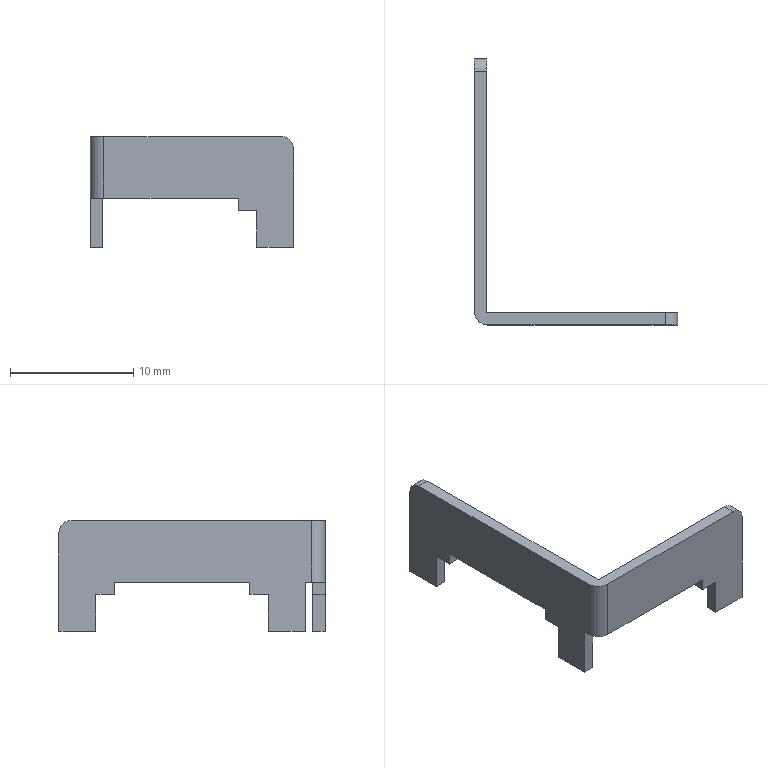Part | STEP file | LRS-150-12_X2_5F00517375-151320 | 1 solid | 26 faces | box 16.5 x 21.6 x 9 mm | volume 224.283 mm3 | plane 22 | cylinder 4 | commonest cylinder face diameters 2 x2 0.2 x1 2.2 x1